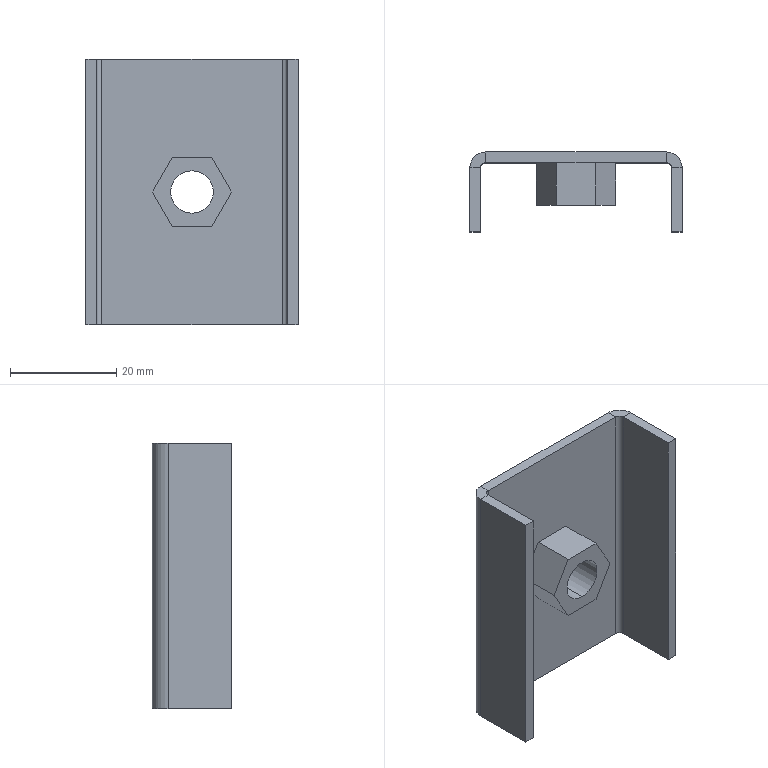Part | SolidWorks | features BaseBody 2 | 2 solids | 34 faces | box 40 x 15 x 50 mm | volume 7052 mm3 | plane 26 | cylinder 8 | commonest cylinder face diameters 2 x2 6 x2 8 x2 9 x2
STEP:
#1=CARTESIAN_POINT('',(0.,-2.,-4.5));
#2=VERTEX_POINT('',#1);
#3=CARTESIAN_POINT('',(0.,0.,-4.5));
#4=VERTEX_POINT('',#3);
#5=CARTESIAN_POINT('',(0.,-2.,-4.5));
#6=DIRECTION('',(0.,1.,0.));
#7=VECTOR('',#6,1000.);
#8=LINE('',#5,#7);
#9=EDGE_CURVE('',#2,#4,#8,.T.);
#10=ORIENTED_EDGE('',*,*,#9,.F.);
#11=CARTESIAN_POINT('',(0.,-2.,4.5));
#12=VERTEX_POINT('',#11);
#13=CARTESIAN_POINT('',(0.,-2.,0.));
#14=DIRECTION('',(0.,1.,0.));
#15=DIRECTION('',(0.,0.,1.));
#16=AXIS2_PLACEMENT_3D('',#13,#14,#15);
#17=CIRCLE('',#16,4.5);
#18=EDGE_CURVE('',#12,#2,#17,.T.);
#19=ORIENTED_EDGE('',*,*,#18,.F.);
#20=CARTESIAN_POINT('',(0.,0.,4.5));
#21=VERTEX_POINT('',#20);
#22=CARTESIAN_POINT('',(0.,-2.,4.5));
#23=DIRECTION('',(0.,1.,0.));
#24=VECTOR('',#23,1000.);
#25=LINE('',#22,#24);
#26=EDGE_CURVE('',#12,#21,#25,.T.);
#27=ORIENTED_EDGE('',*,*,#26,.T.);
#28=CARTESIAN_POINT('',(0.,0.,0.));
#29=DIRECTION('',(0.,1.,0.));
#30=DIRECTION('',(0.,0.,1.));
#31=AXIS2_PLACEMENT_3D('',#28,#29,#30);
#32=CIRCLE('',#31,4.5);
#33=EDGE_CURVE('',#21,#4,#32,.T.);
#34=ORIENTED_EDGE('',*,*,#33,.T.);
#35=EDGE_LOOP('',(#10,#19,#27,#34));
#36=FACE_OUTER_BOUND('',#35,.T.);
#37=CARTESIAN_POINT('',(0.,-2.,0.));
#38=DIRECTION('',(0.,1.,0.));
#39=DIRECTION('',(0.,0.,1.));
#40=AXIS2_PLACEMENT_3D('',#37,#38,#39);
#41=CYLINDRICAL_SURFACE('',#40,4.5);
#42=ADVANCED_FACE('',(#36),#41,.F.);
#43=CARTESIAN_POINT('',(-18.,-15.,25.));
#44=VERTEX_POINT('',#43);
#45=CARTESIAN_POINT('',(-18.,-15.,-25.));
#46=VERTEX_POINT('',#45);
#47=CARTESIAN_POINT('',(-18.,-15.,0.));
#48=DIRECTION('',(0.,0.,-1.));
#49=VECTOR('',#48,1000.);
#50=LINE('',#47,#49);
#51=EDGE_CURVE('',#44,#46,#50,.T.);
#52=ORIENTED_EDGE('',*,*,#51,.F.);
#53=CARTESIAN_POINT('',(-20.,-15.,25.));
#54=VERTEX_POINT('',#53);
#55=CARTESIAN_POINT('',(-20.,-15.,25.));
#56=DIRECTION('',(1.,0.,0.));
#57=VECTOR('',#56,1000.);
#58=LINE('',#55,#57);
#59=EDGE_CURVE('',#54,#44,#58,.T.);
#60=ORIENTED_EDGE('',*,*,#59,.F.);
#61=CARTESIAN_POINT('',(-20.,-15.,-25.));
#62=VERTEX_POINT('',#61);
#63=CARTESIAN_POINT('',(-20.,-15.,25.));
#64=DIRECTION('',(0.,0.,-1.));
#65=VECTOR('',#64,1000.);
#66=LINE('',#63,#65);
#67=EDGE_CURVE('',#54,#62,#66,.T.);
#68=ORIENTED_EDGE('',*,*,#67,.T.);
#69=CARTESIAN_POINT('',(-20.,-15.,-25.));
#70=DIRECTION('',(1.,0.,0.));
#71=VECTOR('',#70,1000.);
#72=LINE('',#69,#71);
#73=EDGE_CURVE('',#62,#46,#72,.T.);
#74=ORIENTED_EDGE('',*,*,#73,.T.);
#75=EDGE_LOOP('',(#52,#60,#68,#74));
#76=FACE_OUTER_BOUND('',#75,.T.);
#77=CARTESIAN_POINT('',(-20.,-15.,25.));
#78=DIRECTION('',(0.,-1.,0.));
#79=DIRECTION('',(-1.,0.,0.));
#80=AXIS2_PLACEMENT_3D('',#77,#78,#79);
#81=PLANE('',#80);
#82=ADVANCED_FACE('',(#76),#81,.T.);
#83=CARTESIAN_POINT('',(-18.,-3.,-25.));
#84=VERTEX_POINT('',#83);
#85=CARTESIAN_POINT('',(-18.,0.,-25.));
#86=DIRECTION('',(0.,1.,0.));
#87=VECTOR('',#86,1000.);
#88=LINE('',#85,#87);
#89=EDGE_CURVE('',#46,#84,#88,.T.);
#90=ORIENTED_EDGE('',*,*,#89,.T.);
#91=CARTESIAN_POINT('',(-18.,-3.,25.));
#92=VERTEX_POINT('',#91);
#93=CARTESIAN_POINT('',(-18.,-3.,25.));
#94=DIRECTION('',(0.,0.,-1.));
#95=VECTOR('',#94,1000.);
#96=LINE('',#93,#95);
#97=EDGE_CURVE('',#92,#84,#96,.T.);
#98=ORIENTED_EDGE('',*,*,#97,.F.);
#99=CARTESIAN_POINT('',(-18.,0.,25.));
#100=DIRECTION('',(0.,-1.,0.));
#101=VECTOR('',#100,1000.);
#102=LINE('',#99,#101);
#103=EDGE_CURVE('',#92,#44,#102,.T.);
#104=ORIENTED_EDGE('',*,*,#103,.T.);
#105=ORIENTED_EDGE('',*,*,#51,.T.);
#106=EDGE_LOOP('',(#90,#98,#104,#105));
#107=FACE_OUTER_BOUND('',#106,.T.);
#108=CARTESIAN_POINT('',(-18.,0.,0.));
#109=DIRECTION('',(1.,0.,0.));
#110=DIRECTION('',(0.,-1.,0.));
#111=AXIS2_PLACEMENT_3D('',#108,#109,#110);
#112=PLANE('',#111);
#113=ADVANCED_FACE('',(#107),#112,.T.);
#114=CARTESIAN_POINT('',(-20.,-3.,-25.));
#115=VERTEX_POINT('',#114);
#116=CARTESIAN_POINT('',(-20.,-3.,25.));
#117=VERTEX_POINT('',#116);
#118=CARTESIAN_POINT('',(-20.,-3.,25.));
#119=DIRECTION('',(0.,0.,1.));
#120=VECTOR('',#119,1000.);
#121=LINE('',#118,#120);
#122=EDGE_CURVE('',#115,#117,#121,.T.);
#123=ORIENTED_EDGE('',*,*,#122,.F.);
#124=CARTESIAN_POINT('',(-20.,-15.,-25.));
#125=DIRECTION('',(0.,1.,0.));
#126=VECTOR('',#125,1000.);
#127=LINE('',#124,#126);
#128=EDGE_CURVE('',#62,#115,#127,.T.);
#129=ORIENTED_EDGE('',*,*,#128,.F.);
#130=ORIENTED_EDGE('',*,*,#67,.F.);
#131=CARTESIAN_POINT('',(-20.,-2.,25.));
#132=DIRECTION('',(0.,-1.,0.));
#133=VECTOR('',#132,1000.);
#134=LINE('',#131,#133);
#135=EDGE_CURVE('',#117,#54,#134,.T.);
#136=ORIENTED_EDGE('',*,*,#135,.F.);
#137=EDGE_LOOP('',(#123,#129,#130,#136));
#138=FACE_OUTER_BOUND('',#137,.T.);
#139=CARTESIAN_POINT('',(-20.,0.,0.));
#140=DIRECTION('',(1.,0.,0.));
#141=DIRECTION('',(0.,-1.,0.));
#142=AXIS2_PLACEMENT_3D('',#139,#140,#141);
#143=PLANE('',#142);
#144=ADVANCED_FACE('',(#138),#143,.F.);
#145=ORIENTED_EDGE('',*,*,#128,.T.);
#146=CARTESIAN_POINT('',(-18.,-3.,-25.));
#147=DIRECTION('',(-1.,0.,0.));
#148=VECTOR('',#147,1000.);
#149=LINE('',#146,#148);
#150=EDGE_CURVE('',#84,#115,#149,.T.);
#151=ORIENTED_EDGE('',*,*,#150,.F.);
#152=ORIENTED_EDGE('',*,*,#89,.F.);
#153=ORIENTED_EDGE('',*,*,#73,.F.);
#154=EDGE_LOOP('',(#145,#151,#152,#153));
#155=FACE_OUTER_BOUND('',#154,.T.);
#156=CARTESIAN_POINT('',(-20.,-15.,-25.));
#157=DIRECTION('',(0.,0.,-1.));
#158=DIRECTION('',(-1.,0.,0.));
#159=AXIS2_PLACEMENT_3D('',#156,#157,#158);
#160=PLANE('',#159);
#161=ADVANCED_FACE('',(#155),#160,.T.);
#162=ORIENTED_EDGE('',*,*,#103,.F.);
#163=CARTESIAN_POINT('',(-20.,-3.,25.));
#164=DIRECTION('',(-1.,0.,0.));
#165=VECTOR('',#164,1000.);
#166=LINE('',#163,#165);
#167=EDGE_CURVE('',#92,#117,#166,.T.);
#168=ORIENTED_EDGE('',*,*,#167,.T.);
#169=ORIENTED_EDGE('',*,*,#135,.T.);
#170=ORIENTED_EDGE('',*,*,#59,.T.);
#171=EDGE_LOOP('',(#162,#168,#169,#170));
#172=FACE_OUTER_BOUND('',#171,.T.);
#173=CARTESIAN_POINT('',(-20.,-2.,25.));
#174=DIRECTION('',(0.,0.,1.));
#175=DIRECTION('',(1.,0.,0.));
#176=AXIS2_PLACEMENT_3D('',#173,#174,#175);
#177=PLANE('',#176);
#178=ADVANCED_FACE('',(#172),#177,.T.);
#179=CARTESIAN_POINT('',(-17.,-2.,-25.));
#180=VERTEX_POINT('',#179);
#181=CARTESIAN_POINT('',(-17.,-2.,25.));
#182=VERTEX_POINT('',#181);
#183=CARTESIAN_POINT('',(-17.,-2.,-25.));
#184=DIRECTION('',(0.,0.,1.));
#185=VECTOR('',#184,1000.);
#186=LINE('',#183,#185);
#187=EDGE_CURVE('',#180,#182,#186,.T.);
#188=ORIENTED_EDGE('',*,*,#187,.T.);
#189=CARTESIAN_POINT('',(-17.,-3.,25.));
#190=DIRECTION('',(0.,0.,1.));
#191=DIRECTION('',(-1.,0.,0.));
#192=AXIS2_PLACEMENT_3D('',#189,#190,#191);
#193=CIRCLE('',#192,1.);
#194=EDGE_CURVE('',#182,#92,#193,.T.);
#195=ORIENTED_EDGE('',*,*,#194,.T.);
#196=ORIENTED_EDGE('',*,*,#97,.T.);
#197=CARTESIAN_POINT('',(-17.,-3.,-25.));
#198=DIRECTION('',(0.,0.,-1.));
#199=DIRECTION('',(-1.,0.,0.));
#200=AXIS2_PLACEMENT_3D('',#197,#198,#199);
#201=CIRCLE('',#200,1.);
#202=EDGE_CURVE('',#84,#180,#201,.T.);
#203=ORIENTED_EDGE('',*,*,#202,.T.);
#204=EDGE_LOOP('',(#188,#195,#196,#203));
#205=FACE_OUTER_BOUND('',#204,.T.);
#206=CARTESIAN_POINT('',(-17.,-3.,-25.));
#207=DIRECTION('',(0.,0.,-1.));
#208=DIRECTION('',(-1.,0.,0.));
#209=AXIS2_PLACEMENT_3D('',#206,#207,#208);
#210=CYLINDRICAL_SURFACE('',#209,1.);
#211=ADVANCED_FACE('',(#205),#210,.F.);
#212=CARTESIAN_POINT('',(-17.,0.,-25.));
#213=VERTEX_POINT('',#212);
#214=CARTESIAN_POINT('',(-17.,0.,25.));
#215=VERTEX_POINT('',#214);
#216=CARTESIAN_POINT('',(-17.,0.,-25.));
#217=DIRECTION('',(0.,0.,1.));
#218=VECTOR('',#217,1000.);
#219=LINE('',#216,#218);
#220=EDGE_CURVE('',#213,#215,#219,.T.);
#221=ORIENTED_EDGE('',*,*,#220,.F.);
#222=CARTESIAN_POINT('',(-17.,-3.,-25.));
#223=DIRECTION('',(0.,0.,-1.));
#224=DIRECTION('',(-1.,0.,0.));
#225=AXIS2_PLACEMENT_3D('',#222,#223,#224);
#226=CIRCLE('',#225,3.);
#227=EDGE_CURVE('',#115,#213,#226,.T.);
#228=ORIENTED_EDGE('',*,*,#227,.F.);
#229=ORIENTED_EDGE('',*,*,#122,.T.);
#230=CARTESIAN_POINT('',(-17.,-3.,25.));
#231=DIRECTION('',(0.,0.,1.));
#232=DIRECTION('',(-1.,0.,0.));
#233=AXIS2_PLACEMENT_3D('',#230,#231,#232);
#234=CIRCLE('',#233,3.);
#235=EDGE_CURVE('',#215,#117,#234,.T.);
#236=ORIENTED_EDGE('',*,*,#235,.F.);
#237=EDGE_LOOP('',(#221,#228,#229,#236));
#238=FACE_OUTER_BOUND('',#237,.T.);
#239=CARTESIAN_POINT('',(-17.,-3.,-25.));
#240=DIRECTION('',(0.,0.,-1.));
#241=DIRECTION('',(-1.,0.,0.));
#242=AXIS2_PLACEMENT_3D('',#239,#240,#241);
#243=CYLINDRICAL_SURFACE('',#242,3.);
#244=ADVANCED_FACE('',(#238),#243,.T.);
#245=ORIENTED_EDGE('',*,*,#202,.F.);
#246=ORIENTED_EDGE('',*,*,#150,.T.);
#247=ORIENTED_EDGE('',*,*,#227,.T.);
#248=CARTESIAN_POINT('',(-17.,-2.,-25.));
#249=DIRECTION('',(0.,1.,0.));
#250=VECTOR('',#249,1000.);
#251=LINE('',#248,#250);
#252=EDGE_CURVE('',#180,#213,#251,.T.);
#253=ORIENTED_EDGE('',*,*,#252,.F.);
#254=EDGE_LOOP('',(#245,#246,#247,#253));
#255=FACE_OUTER_BOUND('',#254,.T.);
#256=CARTESIAN_POINT('',(-17.,-3.,-25.));
#257=DIRECTION('',(0.,0.,1.));
#258=DIRECTION('',(1.,0.,0.));
#259=AXIS2_PLACEMENT_3D('',#256,#257,#258);
#260=PLANE('',#259);
#261=ADVANCED_FACE('',(#255),#260,.F.);
#262=ORIENTED_EDGE('',*,*,#167,.F.);
#263=ORIENTED_EDGE('',*,*,#194,.F.);
#264=CARTESIAN_POINT('',(-17.,-2.,25.));
#265=DIRECTION('',(0.,1.,0.));
#266=VECTOR('',#265,1000.);
#267=LINE('',#264,#266);
#268=EDGE_CURVE('',#182,#215,#267,.T.);
#269=ORIENTED_EDGE('',*,*,#268,.T.);
#270=ORIENTED_EDGE('',*,*,#235,.T.);
#271=EDGE_LOOP('',(#262,#263,#269,#270));
#272=FACE_OUTER_BOUND('',#271,.T.);
#273=CARTESIAN_POINT('',(-17.,-3.,25.));
#274=DIRECTION('',(0.,0.,1.));
#275=DIRECTION('',(1.,0.,0.));
#276=AXIS2_PLACEMENT_3D('',#273,#274,#275);
#277=PLANE('',#276);
#278=ADVANCED_FACE('',(#272),#277,.T.);
#279=CARTESIAN_POINT('',(18.,-15.,-25.));
#280=VERTEX_POINT('',#279);
#281=CARTESIAN_POINT('',(18.,-15.,25.));
#282=VERTEX_POINT('',#281);
#283=CARTESIAN_POINT('',(18.,-15.,0.));
#284=DIRECTION('',(0.,0.,1.));
#285=VECTOR('',#284,1000.);
#286=LINE('',#283,#285);
#287=EDGE_CURVE('',#280,#282,#286,.T.);
#288=ORIENTED_EDGE('',*,*,#287,.F.);
#289=CARTESIAN_POINT('',(20.,-15.,-25.));
#290=VERTEX_POINT('',#289);
#291=CARTESIAN_POINT('',(20.,-15.,-25.));
#292=DIRECTION('',(-1.,0.,0.));
#293=VECTOR('',#292,1000.);
#294=LINE('',#291,#293);
#295=EDGE_CURVE('',#290,#280,#294,.T.);
#296=ORIENTED_EDGE('',*,*,#295,.F.);
#297=CARTESIAN_POINT('',(20.,-15.,25.));
#298=VERTEX_POINT('',#297);
#299=CARTESIAN_POINT('',(20.,-15.,-25.));
#300=DIRECTION('',(0.,0.,1.));
#301=VECTOR('',#300,1000.);
#302=LINE('',#299,#301);
#303=EDGE_CURVE('',#290,#298,#302,.T.);
#304=ORIENTED_EDGE('',*,*,#303,.T.);
#305=CARTESIAN_POINT('',(20.,-15.,25.));
#306=DIRECTION('',(-1.,0.,0.));
#307=VECTOR('',#306,1000.);
#308=LINE('',#305,#307);
#309=EDGE_CURVE('',#298,#282,#308,.T.);
#310=ORIENTED_EDGE('',*,*,#309,.T.);
#311=EDGE_LOOP('',(#288,#296,#304,#310));
#312=FACE_OUTER_BOUND('',#311,.T.);
#313=CARTESIAN_POINT('',(20.,-15.,-25.));
#314=DIRECTION('',(0.,-1.,0.));
#315=DIRECTION('',(0.,0.,-1.));
#316=AXIS2_PLACEMENT_3D('',#313,#314,#315);
#317=PLANE('',#316);
#318=ADVANCED_FACE('',(#312),#317,.T.);
#319=CARTESIAN_POINT('',(18.,-3.,25.));
#320=VERTEX_POINT('',#319);
#321=CARTESIAN_POINT('',(18.,0.,25.));
#322=DIRECTION('',(0.,1.,0.));
#323=VECTOR('',#322,1000.);
#324=LINE('',#321,#323);
#325=EDGE_CURVE('',#282,#320,#324,.T.);
#326=ORIENTED_EDGE('',*,*,#325,.T.);
#327=CARTESIAN_POINT('',(18.,-3.,-25.));
#328=VERTEX_POINT('',#327);
#329=CARTESIAN_POINT('',(18.,-3.,-25.));
#330=DIRECTION('',(0.,0.,1.));
#331=VECTOR('',#330,1000.);
#332=LINE('',#329,#331);
#333=EDGE_CURVE('',#328,#320,#332,.T.);
#334=ORIENTED_EDGE('',*,*,#333,.F.);
#335=CARTESIAN_POINT('',(18.,0.,-25.));
#336=DIRECTION('',(0.,-1.,0.));
#337=VECTOR('',#336,1000.);
#338=LINE('',#335,#337);
#339=EDGE_CURVE('',#328,#280,#338,.T.);
#340=ORIENTED_EDGE('',*,*,#339,.T.);
#341=ORIENTED_EDGE('',*,*,#287,.T.);
#342=EDGE_LOOP('',(#326,#334,#340,#341));
#343=FACE_OUTER_BOUND('',#342,.T.);
#344=CARTESIAN_POINT('',(18.,0.,0.));
#345=DIRECTION('',(-1.,0.,0.));
#346=DIRECTION('',(0.,1.,0.));
#347=AXIS2_PLACEMENT_3D('',#344,#345,#346);
#348=PLANE('',#347);
#349=ADVANCED_FACE('',(#343),#348,.T.);
#350=CARTESIAN_POINT('',(20.,-3.,25.));
#351=VERTEX_POINT('',#350);
#352=CARTESIAN_POINT('',(20.,-3.,-25.));
#353=VERTEX_POINT('',#352);
#354=CARTESIAN_POINT('',(20.,-3.,-25.));
#355=DIRECTION('',(0.,0.,-1.));
#356=VECTOR('',#355,1000.);
#357=LINE('',#354,#356);
#358=EDGE_CURVE('',#351,#353,#357,.T.);
#359=ORIENTED_EDGE('',*,*,#358,.F.);
#360=CARTESIAN_POINT('',(20.,-15.,25.));
#361=DIRECTION('',(0.,1.,0.));
#362=VECTOR('',#361,1000.);
#363=LINE('',#360,#362);
#364=EDGE_CURVE('',#298,#351,#363,.T.);
#365=ORIENTED_EDGE('',*,*,#364,.F.);
#366=ORIENTED_EDGE('',*,*,#303,.F.);
#367=CARTESIAN_POINT('',(20.,-2.,-25.));
#368=DIRECTION('',(0.,-1.,0.));
#369=VECTOR('',#368,1000.);
#370=LINE('',#367,#369);
#371=EDGE_CURVE('',#353,#290,#370,.T.);
#372=ORIENTED_EDGE('',*,*,#371,.F.);
#373=EDGE_LOOP('',(#359,#365,#366,#372));
#374=FACE_OUTER_BOUND('',#373,.T.);
#375=CARTESIAN_POINT('',(20.,0.,0.));
#376=DIRECTION('',(-1.,0.,0.));
#377=DIRECTION('',(0.,1.,0.));
#378=AXIS2_PLACEMENT_3D('',#375,#376,#377);
#379=PLANE('',#378);
#380=ADVANCED_FACE('',(#374),#379,.F.);
#381=ORIENTED_EDGE('',*,*,#364,.T.);
#382=CARTESIAN_POINT('',(18.,-3.,25.));
#383=DIRECTION('',(1.,0.,0.));
#384=VECTOR('',#383,1000.);
#385=LINE('',#382,#384);
#386=EDGE_CURVE('',#320,#351,#385,.T.);
#387=ORIENTED_EDGE('',*,*,#386,.F.);
#388=ORIENTED_EDGE('',*,*,#325,.F.);
#389=ORIENTED_EDGE('',*,*,#309,.F.);
#390=EDGE_LOOP('',(#381,#387,#388,#389));
#391=FACE_OUTER_BOUND('',#390,.T.);
#392=CARTESIAN_POINT('',(20.,-15.,25.));
#393=DIRECTION('',(0.,0.,1.));
#394=DIRECTION('',(0.,-1.,0.));
#395=AXIS2_PLACEMENT_3D('',#392,#393,#394);
#396=PLANE('',#395);
#397=ADVANCED_FACE('',(#391),#396,.T.);
#398=ORIENTED_EDGE('',*,*,#339,.F.);
#399=CARTESIAN_POINT('',(20.,-3.,-25.));
#400=DIRECTION('',(1.,0.,0.));
#401=VECTOR('',#400,1000.);
#402=LINE('',#399,#401);
#403=EDGE_CURVE('',#328,#353,#402,.T.);
#404=ORIENTED_EDGE('',*,*,#403,.T.);
#405=ORIENTED_EDGE('',*,*,#371,.T.);
#406=ORIENTED_EDGE('',*,*,#295,.T.);
#407=EDGE_LOOP('',(#398,#404,#405,#406));
#408=FACE_OUTER_BOUND('',#407,.T.);
#409=CARTESIAN_POINT('',(20.,-2.,-25.));
#410=DIRECTION('',(0.,0.,-1.));
#411=DIRECTION('',(-1.,0.,0.));
#412=AXIS2_PLACEMENT_3D('',#409,#410,#411);
#413=PLANE('',#412);
#414=ADVANCED_FACE('',(#408),#413,.T.);
#415=CARTESIAN_POINT('',(17.,-2.,25.));
#416=VERTEX_POINT('',#415);
#417=CARTESIAN_POINT('',(17.,-2.,-25.));
#418=VERTEX_POINT('',#417);
#419=CARTESIAN_POINT('',(17.,-2.,25.));
#420=DIRECTION('',(0.,0.,-1.));
#421=VECTOR('',#420,1000.);
#422=LINE('',#419,#421);
#423=EDGE_CURVE('',#416,#418,#422,.T.);
#424=ORIENTED_EDGE('',*,*,#423,.T.);
#425=CARTESIAN_POINT('',(17.,-3.,-25.));
#426=DIRECTION('',(0.,0.,-1.));
#427=DIRECTION('',(1.,0.,0.));
#428=AXIS2_PLACEMENT_3D('',#425,#426,#427);
#429=CIRCLE('',#428,1.);
#430=EDGE_CURVE('',#418,#328,#429,.T.);
#431=ORIENTED_EDGE('',*,*,#430,.T.);
#432=ORIENTED_EDGE('',*,*,#333,.T.);
#433=CARTESIAN_POINT('',(17.,-3.,25.));
#434=DIRECTION('',(0.,0.,1.));
#435=DIRECTION('',(1.,0.,0.));
#436=AXIS2_PLACEMENT_3D('',#433,#434,#435);
#437=CIRCLE('',#436,1.);
#438=EDGE_CURVE('',#320,#416,#437,.T.);
#439=ORIENTED_EDGE('',*,*,#438,.T.);
#440=EDGE_LOOP('',(#424,#431,#432,#439));
#441=FACE_OUTER_BOUND('',#440,.T.);
#442=CARTESIAN_POINT('',(17.,-3.,25.));
#443=DIRECTION('',(0.,0.,1.));
#444=DIRECTION('',(1.,0.,0.));
#445=AXIS2_PLACEMENT_3D('',#442,#443,#444);
#446=CYLINDRICAL_SURFACE('',#445,1.);
#447=ADVANCED_FACE('',(#441),#446,.F.);
#448=CARTESIAN_POINT('',(17.,0.,25.));
#449=VERTEX_POINT('',#448);
#450=CARTESIAN_POINT('',(17.,0.,-25.));
#451=VERTEX_POINT('',#450);
#452=CARTESIAN_POINT('',(17.,0.,25.));
#453=DIRECTION('',(0.,0.,-1.));
#454=VECTOR('',#453,1000.);
#455=LINE('',#452,#454);
#456=EDGE_CURVE('',#449,#451,#455,.T.);
#457=ORIENTED_EDGE('',*,*,#456,.F.);
#458=CARTESIAN_POINT('',(17.,-3.,25.));
#459=DIRECTION('',(0.,0.,1.));
#460=DIRECTION('',(1.,0.,0.));
#461=AXIS2_PLACEMENT_3D('',#458,#459,#460);
#462=CIRCLE('',#461,3.);
#463=EDGE_CURVE('',#351,#449,#462,.T.);
#464=ORIENTED_EDGE('',*,*,#463,.F.);
#465=ORIENTED_EDGE('',*,*,#358,.T.);
#466=CARTESIAN_POINT('',(17.,-3.,-25.));
#467=DIRECTION('',(0.,0.,-1.));
#468=DIRECTION('',(1.,0.,0.));
#469=AXIS2_PLACEMENT_3D('',#466,#467,#468);
#470=CIRCLE('',#469,3.);
#471=EDGE_CURVE('',#451,#353,#470,.T.);
#472=ORIENTED_EDGE('',*,*,#471,.F.);
#473=EDGE_LOOP('',(#457,#464,#465,#472));
#474=FACE_OUTER_BOUND('',#473,.T.);
#475=CARTESIAN_POINT('',(17.,-3.,25.));
#476=DIRECTION('',(0.,0.,1.));
#477=DIRECTION('',(1.,0.,0.));
#478=AXIS2_PLACEMENT_3D('',#475,#476,#477);
#479=CYLINDRICAL_SURFACE('',#478,3.);
#480=ADVANCED_FACE('',(#474),#479,.T.);
#481=ORIENTED_EDGE('',*,*,#438,.F.);
#482=ORIENTED_EDGE('',*,*,#386,.T.);
#483=ORIENTED_EDGE('',*,*,#463,.T.);
#484=CARTESIAN_POINT('',(17.,-2.,25.));
#485=DIRECTION('',(0.,1.,0.));
#486=VECTOR('',#485,1000.);
#487=LINE('',#484,#486);
#488=EDGE_CURVE('',#416,#449,#487,.T.);
#489=ORIENTED_EDGE('',*,*,#488,.F.);
#490=EDGE_LOOP('',(#481,#482,#483,#489));
#491=FACE_OUTER_BOUND('',#490,.T.);
#492=CARTESIAN_POINT('',(17.,-3.,25.));
#493=DIRECTION('',(0.,0.,-1.));
#494=DIRECTION('',(0.,-1.,0.));
#495=AXIS2_PLACEMENT_3D('',#492,#493,#494);
#496=PLANE('',#495);
#497=ADVANCED_FACE('',(#491),#496,.F.);
#498=ORIENTED_EDGE('',*,*,#403,.F.);
#499=ORIENTED_EDGE('',*,*,#430,.F.);
#500=CARTESIAN_POINT('',(17.,-2.,-25.));
#501=DIRECTION('',(0.,1.,0.));
#502=VECTOR('',#501,1000.);
#503=LINE('',#500,#502);
#504=EDGE_CURVE('',#418,#451,#503,.T.);
#505=ORIENTED_EDGE('',*,*,#504,.T.);
#506=ORIENTED_EDGE('',*,*,#471,.T.);
#507=EDGE_LOOP('',(#498,#499,#505,#506));
#508=FACE_OUTER_BOUND('',#507,.T.);
#509=CARTESIAN_POINT('',(17.,-3.,-25.));
#510=DIRECTION('',(0.,0.,-1.));
#511=DIRECTION('',(0.,-1.,0.));
#512=AXIS2_PLACEMENT_3D('',#509,#510,#511);
#513=PLANE('',#512);
#514=ADVANCED_FACE('',(#508),#513,.T.);
#515=ORIENTED_EDGE('',*,*,#268,.F.);
#516=CARTESIAN_POINT('',(-20.,-2.,25.));
#517=DIRECTION('',(1.,0.,0.));
#518=VECTOR('',#517,1000.);
#519=LINE('',#516,#518);
#520=EDGE_CURVE('',#182,#416,#519,.T.);
#521=ORIENTED_EDGE('',*,*,#520,.T.);
#522=ORIENTED_EDGE('',*,*,#488,.T.);
#523=CARTESIAN_POINT('',(-20.,0.,25.));
#524=DIRECTION('',(1.,0.,0.));
#525=VECTOR('',#524,1000.);
#526=LINE('',#523,#525);
#527=EDGE_CURVE('',#215,#449,#526,.T.);
#528=ORIENTED_EDGE('',*,*,#527,.F.);
#529=EDGE_LOOP('',(#515,#521,#522,#528));
#530=FACE_OUTER_BOUND('',#529,.T.);
#531=CARTESIAN_POINT('',(-20.,-2.,25.));
#532=DIRECTION('',(0.,0.,1.));
#533=DIRECTION('',(1.,0.,0.));
#534=AXIS2_PLACEMENT_3D('',#531,#532,#533);
#535=PLANE('',#534);
#536=ADVANCED_FACE('',(#530),#535,.T.);
#537=CARTESIAN_POINT('',(-20.,-2.,-25.));
#538=DIRECTION('',(-1.,0.,0.));
#539=VECTOR('',#538,1000.);
#540=LINE('',#537,#539);
#541=EDGE_CURVE('',#418,#180,#540,.T.);
#542=ORIENTED_EDGE('',*,*,#541,.T.);
#543=ORIENTED_EDGE('',*,*,#252,.T.);
#544=CARTESIAN_POINT('',(-20.,0.,-25.));
#545=DIRECTION('',(-1.,0.,0.));
#546=VECTOR('',#545,1000.);
#547=LINE('',#544,#546);
#548=EDGE_CURVE('',#451,#213,#547,.T.);
#549=ORIENTED_EDGE('',*,*,#548,.F.);
#550=ORIENTED_EDGE('',*,*,#504,.F.);
#551=EDGE_LOOP('',(#542,#543,#549,#550));
#552=FACE_OUTER_BOUND('',#551,.T.);
#553=CARTESIAN_POINT('',(-20.,-2.,-25.));
#554=DIRECTION('',(0.,0.,-1.));
#555=DIRECTION('',(0.,-1.,0.));
#556=AXIS2_PLACEMENT_3D('',#553,#554,#555);
#557=PLANE('',#556);
#558=ADVANCED_FACE('',(#552),#557,.T.);
#559=ORIENTED_EDGE('',*,*,#33,.F.);
#560=CARTESIAN_POINT('',(0.,0.,0.));
#561=DIRECTION('',(0.,1.,0.));
#562=DIRECTION('',(0.,0.,1.));
#563=AXIS2_PLACEMENT_3D('',#560,#561,#562);
#564=CIRCLE('',#563,4.5);
#565=EDGE_CURVE('',#4,#21,#564,.T.);
#566=ORIENTED_EDGE('',*,*,#565,.F.);
#567=EDGE_LOOP('',(#559,#566));
#568=FACE_BOUND('',#567,.T.);
#569=ORIENTED_EDGE('',*,*,#548,.T.);
#570=ORIENTED_EDGE('',*,*,#220,.T.);
#571=ORIENTED_EDGE('',*,*,#527,.T.);
#572=ORIENTED_EDGE('',*,*,#456,.T.);
#573=EDGE_LOOP('',(#569,#570,#571,#572));
#574=FACE_OUTER_BOUND('',#573,.T.);
#575=CARTESIAN_POINT('',(0.,0.,0.));
#576=DIRECTION('',(0.,1.,0.));
#577=DIRECTION('',(1.,0.,0.));
#578=AXIS2_PLACEMENT_3D('',#575,#576,#577);
#579=PLANE('',#578);
#580=ADVANCED_FACE('',(#568,#574),#579,.T.);
#581=ORIENTED_EDGE('',*,*,#18,.T.);
#582=CARTESIAN_POINT('',(0.,-2.,0.));
#583=DIRECTION('',(0.,1.,0.));
#584=DIRECTION('',(0.,0.,1.));
#585=AXIS2_PLACEMENT_3D('',#582,#583,#584);
#586=CIRCLE('',#585,4.5);
#587=EDGE_CURVE('',#2,#12,#586,.T.);
#588=ORIENTED_EDGE('',*,*,#587,.T.);
#589=EDGE_LOOP('',(#581,#588));
#590=FACE_BOUND('',#589,.T.);
#591=ORIENTED_EDGE('',*,*,#187,.F.);
#592=ORIENTED_EDGE('',*,*,#541,.F.);
#593=ORIENTED_EDGE('',*,*,#423,.F.);
#594=ORIENTED_EDGE('',*,*,#520,.F.);
#595=EDGE_LOOP('',(#591,#592,#593,#594));
#596=FACE_OUTER_BOUND('',#595,.T.);
#597=CARTESIAN_POINT('',(0.,-2.,0.));
#598=DIRECTION('',(0.,1.,0.));
#599=DIRECTION('',(1.,0.,0.));
#600=AXIS2_PLACEMENT_3D('',#597,#598,#599);
#601=PLANE('',#600);
#602=ADVANCED_FACE('',(#590,#596),#601,.F.);
#603=ORIENTED_EDGE('',*,*,#587,.F.);
#604=ORIENTED_EDGE('',*,*,#9,.T.);
#605=ORIENTED_EDGE('',*,*,#565,.T.);
#606=ORIENTED_EDGE('',*,*,#26,.F.);
#607=EDGE_LOOP('',(#603,#604,#605,#606));
#608=FACE_OUTER_BOUND('',#607,.T.);
#609=CARTESIAN_POINT('',(0.,-2.,0.));
#610=DIRECTION('',(0.,1.,0.));
#611=DIRECTION('',(0.,0.,1.));
#612=AXIS2_PLACEMENT_3D('',#609,#610,#611);
#613=CYLINDRICAL_SURFACE('',#612,4.5);
#614=ADVANCED_FACE('',(#608),#613,.F.);
#615=CLOSED_SHELL('',(#42,#82,#113,#144,#161,#178,#211,#244,#261,#278,#318,#349,#380,#397,#414,#447,#480,#497,#514,#536,#558,#580,#602,#614));
#616=MANIFOLD_SOLID_BREP('',#615);
#617=CARTESIAN_POINT('',(0.,-10.,-4.));
#618=VERTEX_POINT('',#617);
#619=CARTESIAN_POINT('',(0.,-2.,-4.));
#620=VERTEX_POINT('',#619);
#621=CARTESIAN_POINT('',(0.,-10.,-4.));
#622=DIRECTION('',(0.,1.,0.));
#623=VECTOR('',#622,1000.);
#624=LINE('',#621,#623);
#625=EDGE_CURVE('',#618,#620,#624,.T.);
#626=ORIENTED_EDGE('',*,*,#625,.F.);
#627=CARTESIAN_POINT('',(0.,-10.,4.));
#628=VERTEX_POINT('',#627);
#629=CARTESIAN_POINT('',(0.,-10.,0.));
#630=DIRECTION('',(0.,-1.,0.));
#631=DIRECTION('',(0.,0.,-1.));
#632=AXIS2_PLACEMENT_3D('',#629,#630,#631);
#633=CIRCLE('',#632,4.);
#634=EDGE_CURVE('',#618,#628,#633,.T.);
#635=ORIENTED_EDGE('',*,*,#634,.T.);
#636=CARTESIAN_POINT('',(0.,-2.,4.));
#637=VERTEX_POINT('',#636);
#638=CARTESIAN_POINT('',(0.,-10.,4.));
#639=DIRECTION('',(0.,1.,0.));
#640=VECTOR('',#639,1000.);
#641=LINE('',#638,#640);
#642=EDGE_CURVE('',#628,#637,#641,.T.);
#643=ORIENTED_EDGE('',*,*,#642,.T.);
#644=CARTESIAN_POINT('',(0.,-2.,0.));
#645=DIRECTION('',(0.,-1.,0.));
#646=DIRECTION('',(0.,0.,-1.));
#647=AXIS2_PLACEMENT_3D('',#644,#645,#646);
#648=CIRCLE('',#647,4.);
#649=EDGE_CURVE('',#620,#637,#648,.T.);
#650=ORIENTED_EDGE('',*,*,#649,.F.);
#651=EDGE_LOOP('',(#626,#635,#643,#650));
#652=FACE_OUTER_BOUND('',#651,.T.);
#653=CARTESIAN_POINT('',(0.,-10.,0.));
#654=DIRECTION('',(0.,1.,0.));
#655=DIRECTION('',(0.,0.,1.));
#656=AXIS2_PLACEMENT_3D('',#653,#654,#655);
#657=CYLINDRICAL_SURFACE('',#656,4.);
#658=ADVANCED_FACE('',(#652),#657,.F.);
#659=CARTESIAN_POINT('',(-3.724,-2.,-6.45));
#660=VERTEX_POINT('',#659);
#661=CARTESIAN_POINT('',(3.724,-2.,-6.45));
#662=VERTEX_POINT('',#661);
#663=CARTESIAN_POINT('',(-3.724,-2.,-6.45));
#664=DIRECTION('',(1.,0.,0.));
#665=VECTOR('',#664,1000.);
#666=LINE('',#663,#665);
#667=EDGE_CURVE('',#660,#662,#666,.T.);
#668=ORIENTED_EDGE('',*,*,#667,.T.);
#669=CARTESIAN_POINT('',(3.724,-10.,-6.45));
#670=VERTEX_POINT('',#669);
#671=CARTESIAN_POINT('',(3.724,-10.,-6.45));
#672=DIRECTION('',(0.,1.,0.));
#673=VECTOR('',#672,1000.);
#674=LINE('',#671,#673);
#675=EDGE_CURVE('',#670,#662,#674,.T.);
#676=ORIENTED_EDGE('',*,*,#675,.F.);
#677=CARTESIAN_POINT('',(-3.724,-10.,-6.45));
#678=VERTEX_POINT('',#677);
#679=CARTESIAN_POINT('',(-3.724,-10.,-6.45));
#680=DIRECTION('',(1.,0.,0.));
#681=VECTOR('',#680,1000.);
#682=LINE('',#679,#681);
#683=EDGE_CURVE('',#678,#670,#682,.T.);
#684=ORIENTED_EDGE('',*,*,#683,.F.);
#685=CARTESIAN_POINT('',(-3.724,-10.,-6.45));
#686=DIRECTION('',(0.,1.,0.));
#687=VECTOR('',#686,1000.);
#688=LINE('',#685,#687);
#689=EDGE_CURVE('',#678,#660,#688,.T.);
#690=ORIENTED_EDGE('',*,*,#689,.T.);
#691=EDGE_LOOP('',(#668,#676,#684,#690));
#692=FACE_OUTER_BOUND('',#691,.T.);
#693=CARTESIAN_POINT('',(-3.724,-10.,-6.45));
#694=DIRECTION('',(0.,0.,1.));
#695=DIRECTION('',(1.,0.,0.));
#696=AXIS2_PLACEMENT_3D('',#693,#694,#695);
#697=PLANE('',#696);
#698=ADVANCED_FACE('',(#692),#697,.F.);
#699=CARTESIAN_POINT('',(-7.448,-2.,0.));
#700=VERTEX_POINT('',#699);
#701=CARTESIAN_POINT('',(-7.448,-2.,0.));
#702=DIRECTION('',(0.5,0.,-0.866));
#703=VECTOR('',#702,1000.);
#704=LINE('',#701,#703);
#705=EDGE_CURVE('',#700,#660,#704,.T.);
#706=ORIENTED_EDGE('',*,*,#705,.T.);
#707=ORIENTED_EDGE('',*,*,#689,.F.);
#708=CARTESIAN_POINT('',(-7.448,-10.,0.));
#709=VERTEX_POINT('',#708);
#710=CARTESIAN_POINT('',(-7.448,-10.,0.));
#711=DIRECTION('',(0.5,0.,-0.866));
#712=VECTOR('',#711,1000.);
#713=LINE('',#710,#712);
#714=EDGE_CURVE('',#709,#678,#713,.T.);
#715=ORIENTED_EDGE('',*,*,#714,.F.);
#716=CARTESIAN_POINT('',(-7.448,-10.,0.));
#717=DIRECTION('',(0.,1.,0.));
#718=VECTOR('',#717,1000.);
#719=LINE('',#716,#718);
#720=EDGE_CURVE('',#709,#700,#719,.T.);
#721=ORIENTED_EDGE('',*,*,#720,.T.);
#722=EDGE_LOOP('',(#706,#707,#715,#721));
#723=FACE_OUTER_BOUND('',#722,.T.);
#724=CARTESIAN_POINT('',(-7.448,-10.,0.));
#725=DIRECTION('',(0.866,0.,0.5));
#726=DIRECTION('',(0.,-1.,0.));
#727=AXIS2_PLACEMENT_3D('',#724,#725,#726);
#728=PLANE('',#727);
#729=ADVANCED_FACE('',(#723),#728,.F.);
#730=CARTESIAN_POINT('',(-3.724,-2.,6.45));
#731=VERTEX_POINT('',#730);
#732=CARTESIAN_POINT('',(-3.724,-2.,6.45));
#733=DIRECTION('',(-0.5,0.,-0.866));
#734=VECTOR('',#733,1000.);
#735=LINE('',#732,#734);
#736=EDGE_CURVE('',#731,#700,#735,.T.);
#737=ORIENTED_EDGE('',*,*,#736,.T.);
#738=ORIENTED_EDGE('',*,*,#720,.F.);
#739=CARTESIAN_POINT('',(-3.724,-10.,6.45));
#740=VERTEX_POINT('',#739);
#741=CARTESIAN_POINT('',(-3.724,-10.,6.45));
#742=DIRECTION('',(-0.5,0.,-0.866));
#743=VECTOR('',#742,1000.);
#744=LINE('',#741,#743);
#745=EDGE_CURVE('',#740,#709,#744,.T.);
#746=ORIENTED_EDGE('',*,*,#745,.F.);
#747=CARTESIAN_POINT('',(-3.724,-10.,6.45));
#748=DIRECTION('',(0.,1.,0.));
#749=VECTOR('',#748,1000.);
#750=LINE('',#747,#749);
#751=EDGE_CURVE('',#740,#731,#750,.T.);
#752=ORIENTED_EDGE('',*,*,#751,.T.);
#753=EDGE_LOOP('',(#737,#738,#746,#752));
#754=FACE_OUTER_BOUND('',#753,.T.);
#755=CARTESIAN_POINT('',(-3.724,-10.,6.45));
#756=DIRECTION('',(0.866,0.,-0.5));
#757=DIRECTION('',(0.,-1.,0.));
#758=AXIS2_PLACEMENT_3D('',#755,#756,#757);
#759=PLANE('',#758);
#760=ADVANCED_FACE('',(#754),#759,.F.);
#761=CARTESIAN_POINT('',(3.724,-2.,6.45));
#762=VERTEX_POINT('',#761);
#763=CARTESIAN_POINT('',(3.724,-2.,6.45));
#764=DIRECTION('',(-1.,0.,0.));
#765=VECTOR('',#764,1000.);
#766=LINE('',#763,#765);
#767=EDGE_CURVE('',#762,#731,#766,.T.);
#768=ORIENTED_EDGE('',*,*,#767,.T.);
#769=ORIENTED_EDGE('',*,*,#751,.F.);
#770=CARTESIAN_POINT('',(3.724,-10.,6.45));
#771=VERTEX_POINT('',#770);
#772=CARTESIAN_POINT('',(3.724,-10.,6.45));
#773=DIRECTION('',(-1.,0.,0.));
#774=VECTOR('',#773,1000.);
#775=LINE('',#772,#774);
#776=EDGE_CURVE('',#771,#740,#775,.T.);
#777=ORIENTED_EDGE('',*,*,#776,.F.);
#778=CARTESIAN_POINT('',(3.724,-10.,6.45));
#779=DIRECTION('',(0.,1.,0.));
#780=VECTOR('',#779,1000.);
#781=LINE('',#778,#780);
#782=EDGE_CURVE('',#771,#762,#781,.T.);
#783=ORIENTED_EDGE('',*,*,#782,.T.);
#784=EDGE_LOOP('',(#768,#769,#777,#783));
#785=FACE_OUTER_BOUND('',#784,.T.);
#786=CARTESIAN_POINT('',(3.724,-10.,6.45));
#787=DIRECTION('',(0.,0.,-1.));
#788=DIRECTION('',(0.,-1.,0.));
#789=AXIS2_PLACEMENT_3D('',#786,#787,#788);
#790=PLANE('',#789);
#791=ADVANCED_FACE('',(#785),#790,.F.);
#792=CARTESIAN_POINT('',(7.448,-2.,0.));
#793=VERTEX_POINT('',#792);
#794=CARTESIAN_POINT('',(7.448,-2.,0.));
#795=DIRECTION('',(-0.5,0.,0.866));
#796=VECTOR('',#795,1000.);
#797=LINE('',#794,#796);
#798=EDGE_CURVE('',#793,#762,#797,.T.);
#799=ORIENTED_EDGE('',*,*,#798,.T.);
#800=ORIENTED_EDGE('',*,*,#782,.F.);
#801=CARTESIAN_POINT('',(7.448,-10.,0.));
#802=VERTEX_POINT('',#801);
#803=CARTESIAN_POINT('',(7.448,-10.,0.));
#804=DIRECTION('',(-0.5,0.,0.866));
#805=VECTOR('',#804,1000.);
#806=LINE('',#803,#805);
#807=EDGE_CURVE('',#802,#771,#806,.T.);
#808=ORIENTED_EDGE('',*,*,#807,.F.);
#809=CARTESIAN_POINT('',(7.448,-10.,0.));
#810=DIRECTION('',(0.,1.,0.));
#811=VECTOR('',#810,1000.);
#812=LINE('',#809,#811);
#813=EDGE_CURVE('',#802,#793,#812,.T.);
#814=ORIENTED_EDGE('',*,*,#813,.T.);
#815=EDGE_LOOP('',(#799,#800,#808,#814));
#816=FACE_OUTER_BOUND('',#815,.T.);
#817=CARTESIAN_POINT('',(7.448,-10.,0.));
#818=DIRECTION('',(-0.866,0.,-0.5));
#819=DIRECTION('',(-0.5,0.,0.866));
#820=AXIS2_PLACEMENT_3D('',#817,#818,#819);
#821=PLANE('',#820);
#822=ADVANCED_FACE('',(#816),#821,.F.);
#823=CARTESIAN_POINT('',(3.724,-2.,-6.45));
#824=DIRECTION('',(0.5,0.,0.866));
#825=VECTOR('',#824,1000.);
#826=LINE('',#823,#825);
#827=EDGE_CURVE('',#662,#793,#826,.T.);
#828=ORIENTED_EDGE('',*,*,#827,.T.);
#829=ORIENTED_EDGE('',*,*,#813,.F.);
#830=CARTESIAN_POINT('',(3.724,-10.,-6.45));
#831=DIRECTION('',(0.5,0.,0.866));
#832=VECTOR('',#831,1000.);
#833=LINE('',#830,#832);
#834=EDGE_CURVE('',#670,#802,#833,.T.);
#835=ORIENTED_EDGE('',*,*,#834,.F.);
#836=ORIENTED_EDGE('',*,*,#675,.T.);
#837=EDGE_LOOP('',(#828,#829,#835,#836));
#838=FACE_OUTER_BOUND('',#837,.T.);
#839=CARTESIAN_POINT('',(3.724,-10.,-6.45));
#840=DIRECTION('',(-0.866,0.,0.5));
#841=DIRECTION('',(0.,1.,0.));
#842=AXIS2_PLACEMENT_3D('',#839,#840,#841);
#843=PLANE('',#842);
#844=ADVANCED_FACE('',(#838),#843,.F.);
#845=CARTESIAN_POINT('',(0.,-2.,0.));
#846=DIRECTION('',(0.,-1.,0.));
#847=DIRECTION('',(0.,0.,-1.));
#848=AXIS2_PLACEMENT_3D('',#845,#846,#847);
#849=CIRCLE('',#848,4.);
#850=EDGE_CURVE('',#637,#620,#849,.T.);
#851=ORIENTED_EDGE('',*,*,#850,.T.);
#852=ORIENTED_EDGE('',*,*,#649,.T.);
#853=EDGE_LOOP('',(#851,#852));
#854=FACE_BOUND('',#853,.T.);
#855=ORIENTED_EDGE('',*,*,#827,.F.);
#856=ORIENTED_EDGE('',*,*,#667,.F.);
#857=ORIENTED_EDGE('',*,*,#705,.F.);
#858=ORIENTED_EDGE('',*,*,#736,.F.);
#859=ORIENTED_EDGE('',*,*,#767,.F.);
#860=ORIENTED_EDGE('',*,*,#798,.F.);
#861=EDGE_LOOP('',(#855,#856,#857,#858,#859,#860));
#862=FACE_OUTER_BOUND('',#861,.T.);
#863=CARTESIAN_POINT('',(0.,-2.,0.));
#864=DIRECTION('',(0.,-1.,0.));
#865=DIRECTION('',(0.,0.,-1.));
#866=AXIS2_PLACEMENT_3D('',#863,#864,#865);
#867=PLANE('',#866);
#868=ADVANCED_FACE('',(#854,#862),#867,.F.);
#869=CARTESIAN_POINT('',(0.,-10.,0.));
#870=DIRECTION('',(0.,-1.,0.));
#871=DIRECTION('',(0.,0.,-1.));
#872=AXIS2_PLACEMENT_3D('',#869,#870,#871);
#873=CIRCLE('',#872,4.);
#874=EDGE_CURVE('',#628,#618,#873,.T.);
#875=ORIENTED_EDGE('',*,*,#874,.F.);
#876=ORIENTED_EDGE('',*,*,#634,.F.);
#877=EDGE_LOOP('',(#875,#876));
#878=FACE_BOUND('',#877,.T.);
#879=ORIENTED_EDGE('',*,*,#834,.T.);
#880=ORIENTED_EDGE('',*,*,#807,.T.);
#881=ORIENTED_EDGE('',*,*,#776,.T.);
#882=ORIENTED_EDGE('',*,*,#745,.T.);
#883=ORIENTED_EDGE('',*,*,#714,.T.);
#884=ORIENTED_EDGE('',*,*,#683,.T.);
#885=EDGE_LOOP('',(#879,#880,#881,#882,#883,#884));
#886=FACE_OUTER_BOUND('',#885,.T.);
#887=CARTESIAN_POINT('',(0.,-10.,0.));
#888=DIRECTION('',(0.,-1.,0.));
#889=DIRECTION('',(0.,0.,-1.));
#890=AXIS2_PLACEMENT_3D('',#887,#888,#889);
#891=PLANE('',#890);
#892=ADVANCED_FACE('',(#878,#886),#891,.T.);
#893=ORIENTED_EDGE('',*,*,#874,.T.);
#894=ORIENTED_EDGE('',*,*,#625,.T.);
#895=ORIENTED_EDGE('',*,*,#850,.F.);
#896=ORIENTED_EDGE('',*,*,#642,.F.);
#897=EDGE_LOOP('',(#893,#894,#895,#896));
#898=FACE_OUTER_BOUND('',#897,.T.);
#899=CARTESIAN_POINT('',(0.,-10.,0.));
#900=DIRECTION('',(0.,1.,0.));
#901=DIRECTION('',(0.,0.,1.));
#902=AXIS2_PLACEMENT_3D('',#899,#900,#901);
#903=CYLINDRICAL_SURFACE('',#902,4.);
#904=ADVANCED_FACE('',(#898),#903,.F.);
#905=CLOSED_SHELL('',(#658,#698,#729,#760,#791,#822,#844,#868,#892,#904));
#906=MANIFOLD_SOLID_BREP('',#905);
#907=CARTESIAN_POINT('',(0.,0.,0.));
#908=DIRECTION('',(0.,0.,1.));
#909=DIRECTION('',(1.,0.,0.));
#910=AXIS2_PLACEMENT_3D('',#907,#908,#909);
#911=(LENGTH_UNIT()NAMED_UNIT(*)SI_UNIT(.MILLI.,.METRE.));
#912=UNCERTAINTY_MEASURE_WITH_UNIT(LENGTH_MEASURE(0.00001),#911,'','');
#913=(NAMED_UNIT(*)PLANE_ANGLE_UNIT()SI_UNIT($,.RADIAN.));
#914=(NAMED_UNIT(*)SI_UNIT($,.STERADIAN.)SOLID_ANGLE_UNIT());
#915=(GEOMETRIC_REPRESENTATION_CONTEXT(3)GLOBAL_UNCERTAINTY_ASSIGNED_CONTEXT((#912))GLOBAL_UNIT_ASSIGNED_CONTEXT((#911,#913,#914))REPRESENTATION_CONTEXT('',''));
#916=ADVANCED_BREP_SHAPE_REPRESENTATION('',(#616,#906,#910),#915);